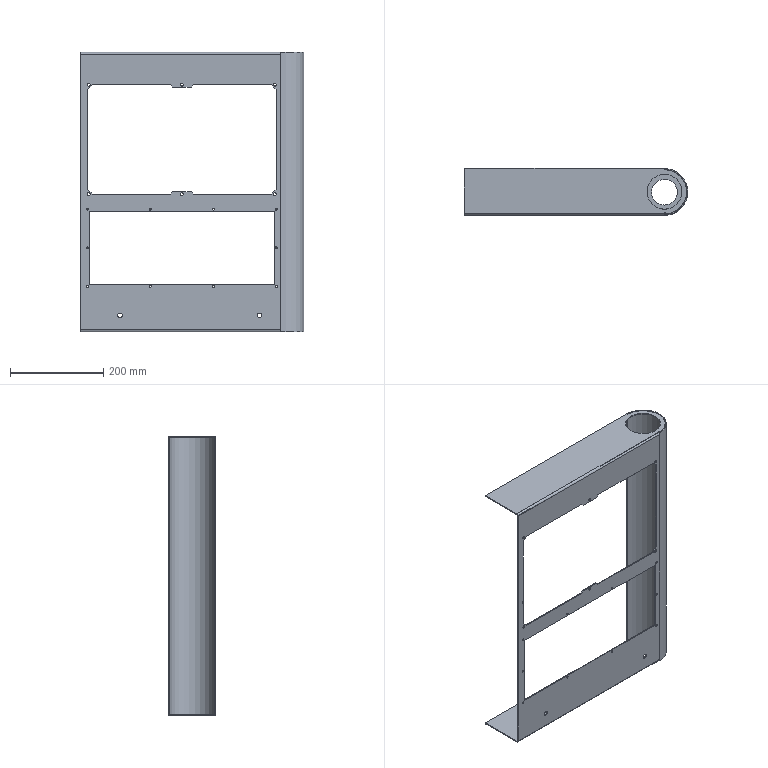Part | NX | features solid 2 | 1 solid | 104 faces | box 480 x 100 x 600 mm | volume 551703 mm3 | cylinder 54 | plane 50 | commonest cylinder face diameters 4 x22 6 x14 10 x4 55.2 x3 95 x3 8 x2